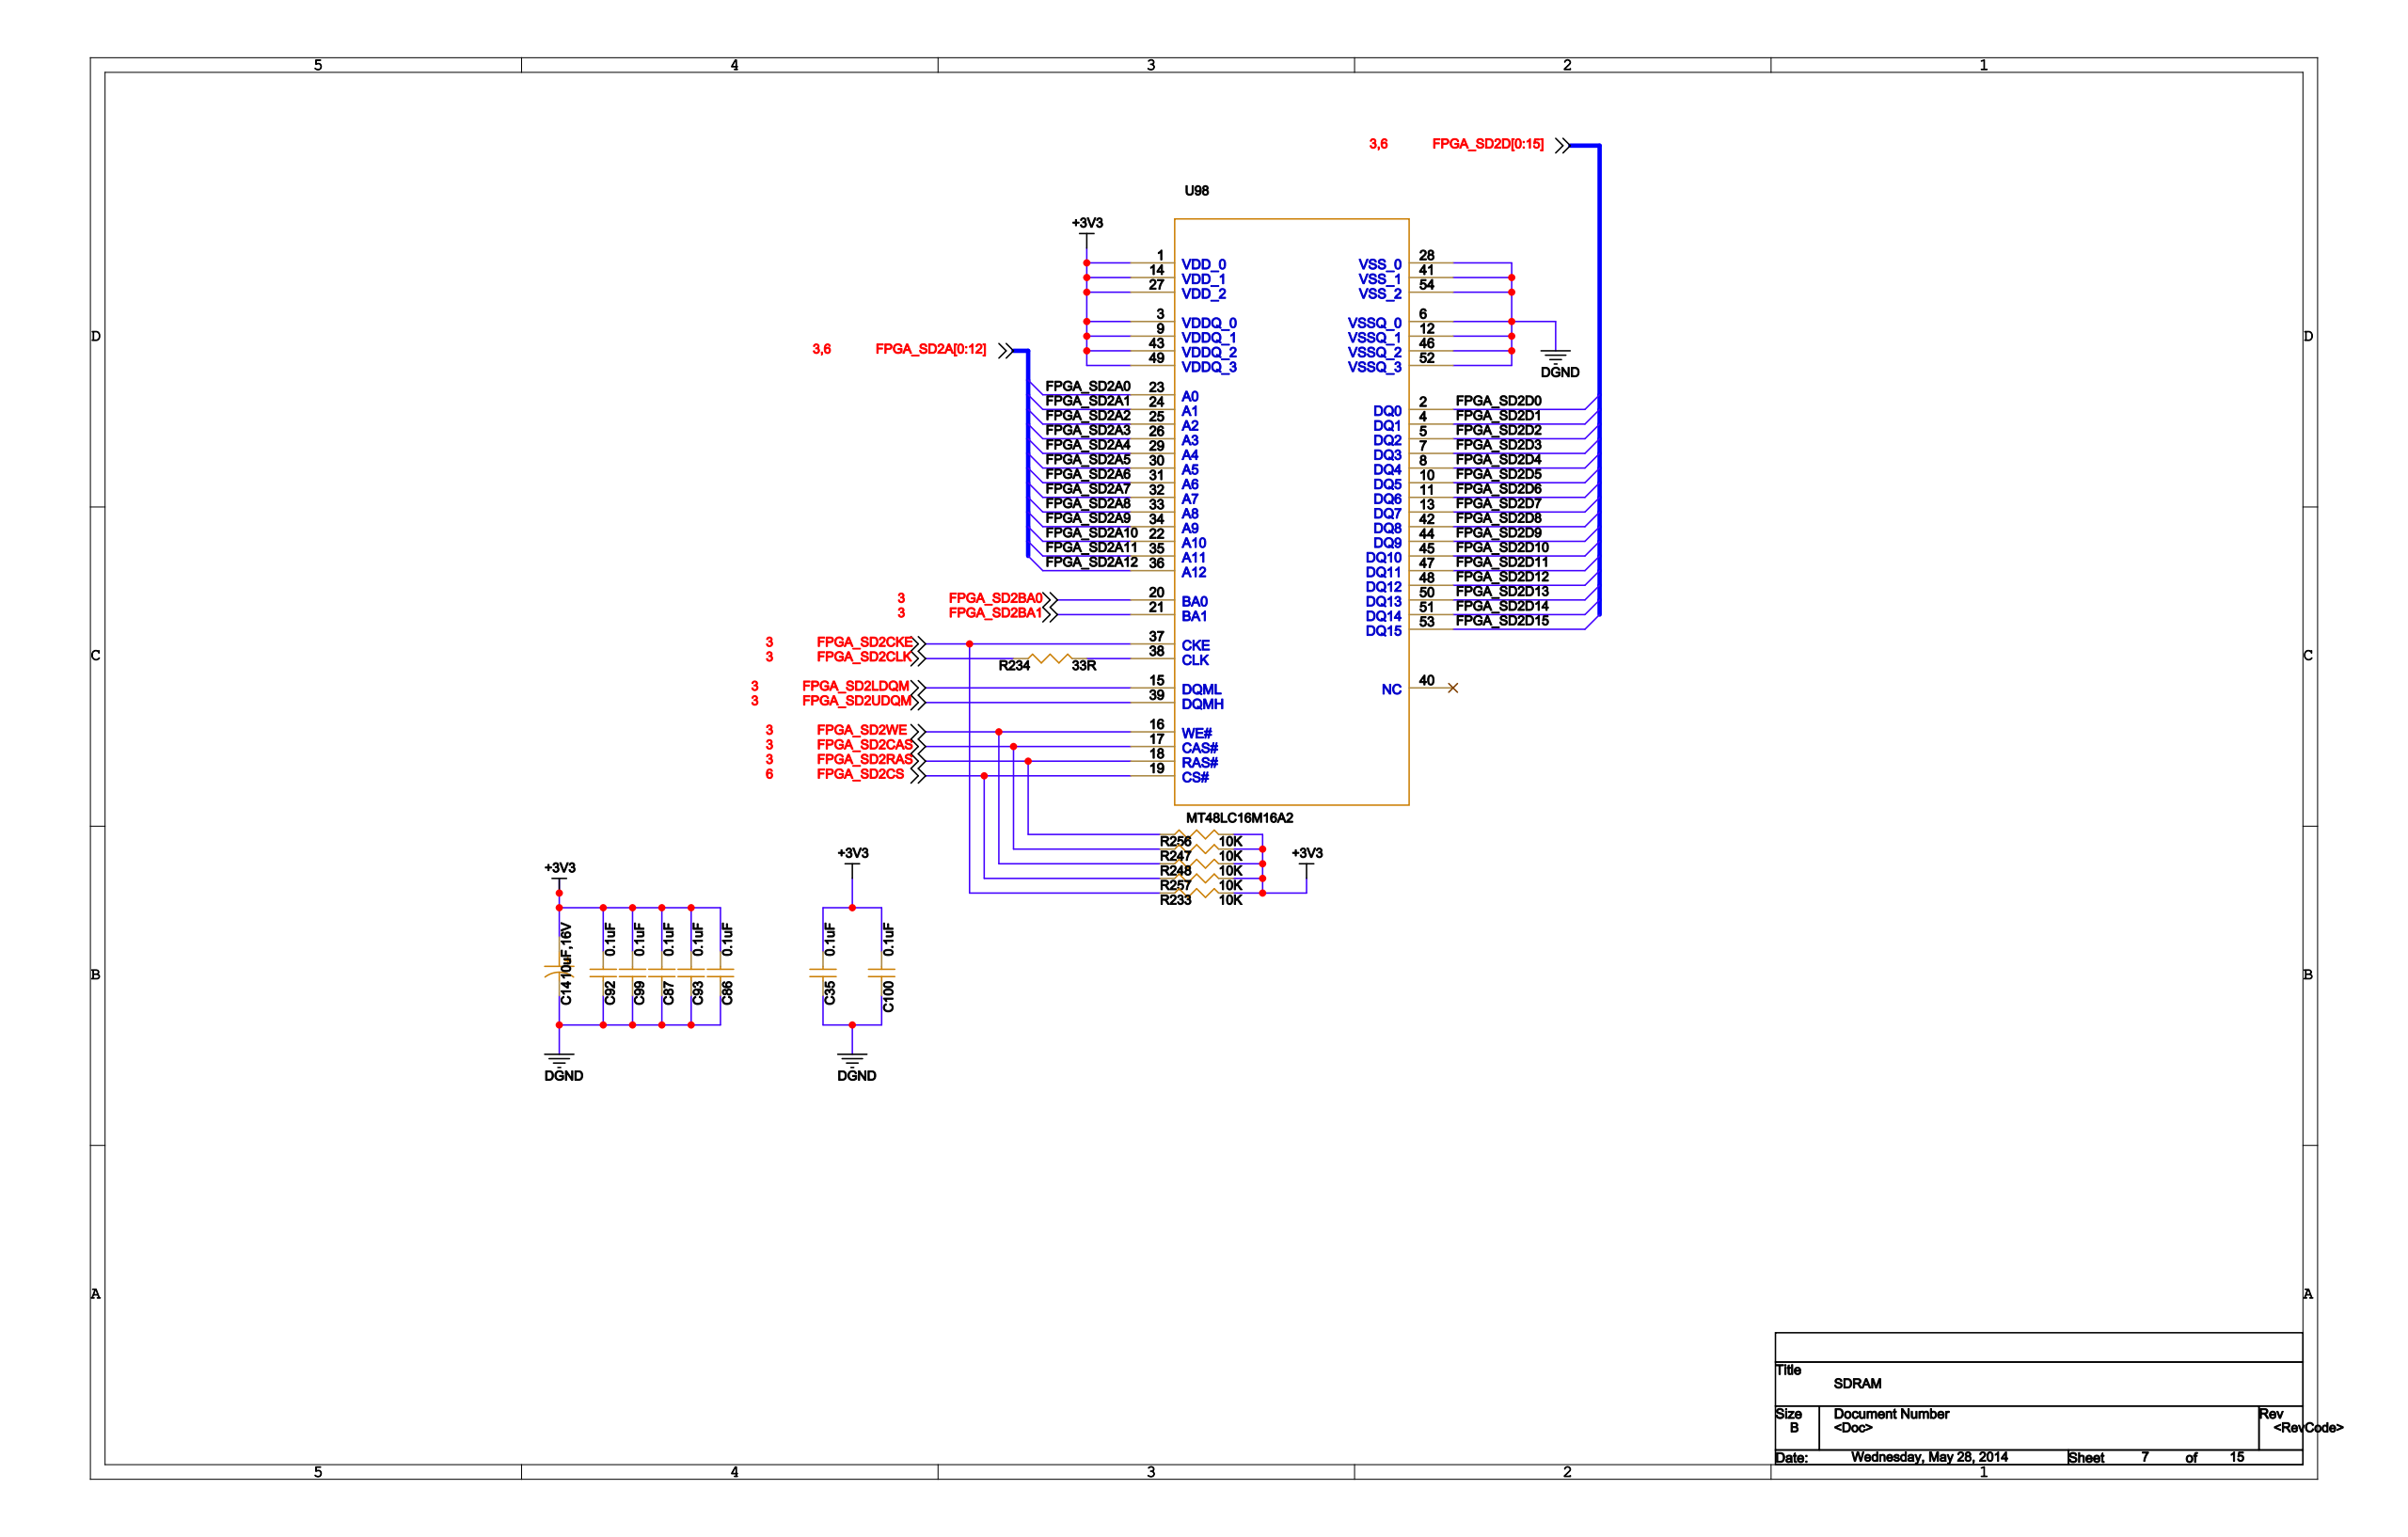Circuit board | Cadence Allegro | 669 parts | 806 nets | one sheet of the schematic
Parts on this sheet (reference | value | footprint):
C35 | 0.1uF | C0402
C86 | 0.1uF | C0402
C87 | 0.1uF | C0402
C92 | 0.1uF | C0402
C93 | 0.1uF | C0402
C99 | 0.1uF | C0402
C100 | 0.1uF | C0402
R233 | 10K | R0603
R234 | 33R | R0603
R247 | 10K | R0603
R248 | 10K | R0603
R256 | 10K | R0603
R257 | 10K | R0603
U98 | MT48LC16M16A2 | TSOP54
Nets of these parts (net: part-pin ...):
DGND: C35-2 C86-2 C87-2 C92-2 C93-2 C99-2 C100-2 U98-6 U98-12 U98-28 U98-41 U98-46 U98-52 U98-54
+3V3: C35-1 C86-1 C87-1 C92-1 C93-1 C99-1 C100-1 R233-2 R247-2 R248-2 R256-2 R257-2 U98-1 U98-3 U98-9 U98-14 U98-27 U98-43 U98-49
FPGA_SD2CS: R257-1 U98-19
FPGA_SD2D13: U98-50
FPGA_SD2A6: U98-31
FPGA_SD2D6: U98-11
FPGA_SD2D7: U98-13
FPGA_SD2RAS: R256-1 U98-18
FPGA_SD2LDQM: U98-15
FPGA_SD2WE: R248-1 U98-16
FPGA_SD2D0: U98-2
FPGA_SD2D2: U98-5
FPGA_SD2D4: U98-8
FPGA_SD2D1: U98-4
FPGA_SD2D3: U98-7
FPGA_SD2D5: U98-10
FPGA_SD2A1: U98-24
FPGA_SD2CAS: R247-1 U98-17
FPGA_SD2CLK: R234-1
FPGA_SD2A12: U98-36
FPGA_SD2BA1: U98-21
FPGA_SD2D10: U98-45
FPGA_SD2D12: U98-48
FPGA_SD2D14: U98-51
FPGA_SD2D11: U98-47
FPGA_SD2D15: U98-53
FPGA_SD2A4: U98-29
FPGA_SD2CKE: R233-1 U98-37
FPGA_SD2A8: U98-33
FPGA_SD2D9: U98-44
FPGA_SD2BA0: U98-20
FPGA_SD2A3: U98-26
FPGA_SD2A10: U98-22
FPGA_SD2A11: U98-35
FPGA_SD2A0: U98-23
FPGA_SD2A7: U98-32
FPGA_SD2A9: U98-34
FPGA_SD2UDQM: U98-39
FPGA_SD2D8: U98-42
FPGA_SD2A5: U98-30
FPGA_SD2A2: U98-25
N61323521: R234-2 U98-38